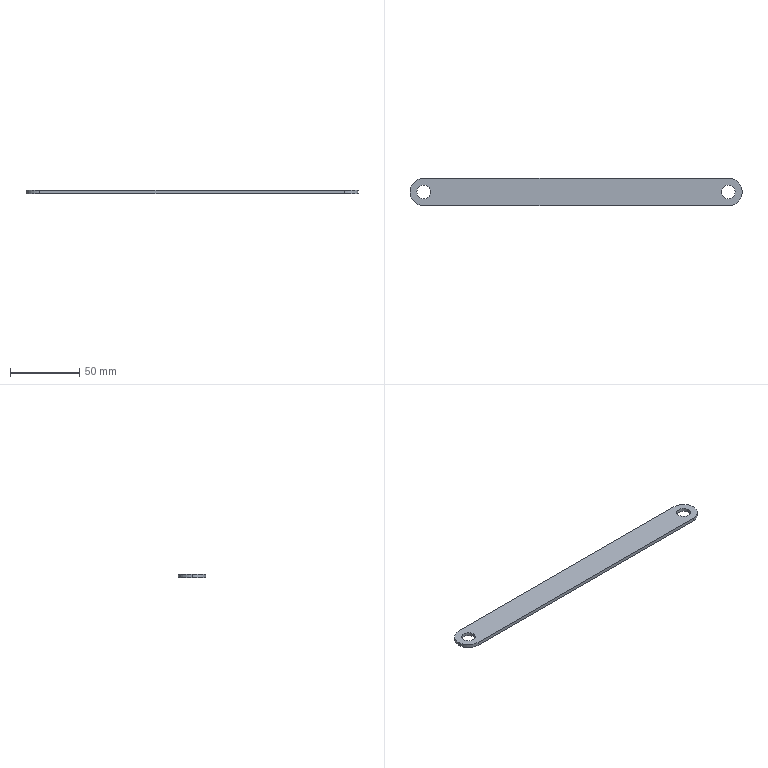Part | SolidWorks | features Extrusion 1 | 1 solid | 11 faces | box 240 x 20 x 2.5 mm | volume 11393 mm3 | cylinder 7 | plane 4 | commonest cylinder face diameters 10 x4 20 x3
STEP:
#1=CARTESIAN_POINT('',(105.,0.,2.5));
#2=VERTEX_POINT('',#1);
#3=CARTESIAN_POINT('',(115.,0.,2.5));
#4=VERTEX_POINT('',#3);
#5=CARTESIAN_POINT('',(110.,0.,2.5));
#6=DIRECTION('',(0.,0.,1.));
#7=DIRECTION('',(1.,0.,0.));
#8=AXIS2_PLACEMENT_3D('',#5,#6,#7);
#9=CIRCLE('',#8,5.);
#10=EDGE_CURVE('',#2,#4,#9,.T.);
#11=ORIENTED_EDGE('',*,*,#10,.T.);
#12=CARTESIAN_POINT('',(115.,0.,0.));
#13=VERTEX_POINT('',#12);
#14=CARTESIAN_POINT('',(115.,0.,2.5));
#15=DIRECTION('',(0.,0.,-1.));
#16=VECTOR('',#15,1000.);
#17=LINE('',#14,#16);
#18=EDGE_CURVE('',#4,#13,#17,.T.);
#19=ORIENTED_EDGE('',*,*,#18,.T.);
#20=CARTESIAN_POINT('',(105.,0.,0.));
#21=VERTEX_POINT('',#20);
#22=CARTESIAN_POINT('',(110.,0.,0.));
#23=DIRECTION('',(0.,0.,1.));
#24=DIRECTION('',(1.,0.,0.));
#25=AXIS2_PLACEMENT_3D('',#22,#23,#24);
#26=CIRCLE('',#25,5.);
#27=EDGE_CURVE('',#21,#13,#26,.T.);
#28=ORIENTED_EDGE('',*,*,#27,.F.);
#29=CARTESIAN_POINT('',(105.,0.,2.5));
#30=DIRECTION('',(0.,0.,-1.));
#31=VECTOR('',#30,1000.);
#32=LINE('',#29,#31);
#33=EDGE_CURVE('',#2,#21,#32,.T.);
#34=ORIENTED_EDGE('',*,*,#33,.F.);
#35=EDGE_LOOP('',(#11,#19,#28,#34));
#36=FACE_OUTER_BOUND('',#35,.T.);
#37=CARTESIAN_POINT('',(110.,0.,2.5));
#38=DIRECTION('',(0.,0.,-1.));
#39=DIRECTION('',(-1.,0.,0.));
#40=AXIS2_PLACEMENT_3D('',#37,#38,#39);
#41=CYLINDRICAL_SURFACE('',#40,5.);
#42=ADVANCED_FACE('',(#36),#41,.F.);
#43=CARTESIAN_POINT('',(-115.,0.,2.5));
#44=VERTEX_POINT('',#43);
#45=CARTESIAN_POINT('',(-105.,0.,2.5));
#46=VERTEX_POINT('',#45);
#47=CARTESIAN_POINT('',(-110.,0.,2.5));
#48=DIRECTION('',(0.,0.,1.));
#49=DIRECTION('',(1.,0.,0.));
#50=AXIS2_PLACEMENT_3D('',#47,#48,#49);
#51=CIRCLE('',#50,5.);
#52=EDGE_CURVE('',#44,#46,#51,.T.);
#53=ORIENTED_EDGE('',*,*,#52,.T.);
#54=CARTESIAN_POINT('',(-105.,0.,0.));
#55=VERTEX_POINT('',#54);
#56=CARTESIAN_POINT('',(-105.,0.,2.5));
#57=DIRECTION('',(0.,0.,-1.));
#58=VECTOR('',#57,1000.);
#59=LINE('',#56,#58);
#60=EDGE_CURVE('',#46,#55,#59,.T.);
#61=ORIENTED_EDGE('',*,*,#60,.T.);
#62=CARTESIAN_POINT('',(-115.,0.,0.));
#63=VERTEX_POINT('',#62);
#64=CARTESIAN_POINT('',(-110.,0.,0.));
#65=DIRECTION('',(0.,0.,1.));
#66=DIRECTION('',(1.,0.,0.));
#67=AXIS2_PLACEMENT_3D('',#64,#65,#66);
#68=CIRCLE('',#67,5.);
#69=EDGE_CURVE('',#63,#55,#68,.T.);
#70=ORIENTED_EDGE('',*,*,#69,.F.);
#71=CARTESIAN_POINT('',(-115.,0.,2.5));
#72=DIRECTION('',(0.,0.,-1.));
#73=VECTOR('',#72,1000.);
#74=LINE('',#71,#73);
#75=EDGE_CURVE('',#44,#63,#74,.T.);
#76=ORIENTED_EDGE('',*,*,#75,.F.);
#77=EDGE_LOOP('',(#53,#61,#70,#76));
#78=FACE_OUTER_BOUND('',#77,.T.);
#79=CARTESIAN_POINT('',(-110.,0.,2.5));
#80=DIRECTION('',(0.,0.,-1.));
#81=DIRECTION('',(-1.,0.,0.));
#82=AXIS2_PLACEMENT_3D('',#79,#80,#81);
#83=CYLINDRICAL_SURFACE('',#82,5.);
#84=ADVANCED_FACE('',(#78),#83,.F.);
#85=CARTESIAN_POINT('',(-120.,0.,2.5));
#86=VERTEX_POINT('',#85);
#87=CARTESIAN_POINT('',(-110.,-10.,2.5));
#88=VERTEX_POINT('',#87);
#89=CARTESIAN_POINT('',(-110.,0.,2.5));
#90=DIRECTION('',(0.,0.,1.));
#91=DIRECTION('',(1.,0.,0.));
#92=AXIS2_PLACEMENT_3D('',#89,#90,#91);
#93=CIRCLE('',#92,10.);
#94=EDGE_CURVE('',#86,#88,#93,.T.);
#95=ORIENTED_EDGE('',*,*,#94,.F.);
#96=CARTESIAN_POINT('',(-120.,0.,0.));
#97=VERTEX_POINT('',#96);
#98=CARTESIAN_POINT('',(-120.,0.,2.5));
#99=DIRECTION('',(0.,0.,-1.));
#100=VECTOR('',#99,1000.);
#101=LINE('',#98,#100);
#102=EDGE_CURVE('',#86,#97,#101,.T.);
#103=ORIENTED_EDGE('',*,*,#102,.T.);
#104=CARTESIAN_POINT('',(-110.,-10.,0.));
#105=VERTEX_POINT('',#104);
#106=CARTESIAN_POINT('',(-110.,0.,0.));
#107=DIRECTION('',(0.,0.,1.));
#108=DIRECTION('',(1.,0.,0.));
#109=AXIS2_PLACEMENT_3D('',#106,#107,#108);
#110=CIRCLE('',#109,10.);
#111=EDGE_CURVE('',#97,#105,#110,.T.);
#112=ORIENTED_EDGE('',*,*,#111,.T.);
#113=CARTESIAN_POINT('',(-110.,-10.,2.5));
#114=DIRECTION('',(0.,0.,-1.));
#115=VECTOR('',#114,1000.);
#116=LINE('',#113,#115);
#117=EDGE_CURVE('',#88,#105,#116,.T.);
#118=ORIENTED_EDGE('',*,*,#117,.F.);
#119=EDGE_LOOP('',(#95,#103,#112,#118));
#120=FACE_OUTER_BOUND('',#119,.T.);
#121=CARTESIAN_POINT('',(-110.,0.,2.5));
#122=DIRECTION('',(0.,0.,-1.));
#123=DIRECTION('',(-1.,0.,0.));
#124=AXIS2_PLACEMENT_3D('',#121,#122,#123);
#125=CYLINDRICAL_SURFACE('',#124,10.);
#126=ADVANCED_FACE('',(#120),#125,.T.);
#127=ORIENTED_EDGE('',*,*,#52,.F.);
#128=CARTESIAN_POINT('',(-110.,0.,2.5));
#129=DIRECTION('',(0.,0.,1.));
#130=DIRECTION('',(1.,0.,0.));
#131=AXIS2_PLACEMENT_3D('',#128,#129,#130);
#132=CIRCLE('',#131,5.);
#133=EDGE_CURVE('',#46,#44,#132,.T.);
#134=ORIENTED_EDGE('',*,*,#133,.F.);
#135=EDGE_LOOP('',(#127,#134));
#136=FACE_BOUND('',#135,.T.);
#137=CARTESIAN_POINT('',(-110.,10.,2.5));
#138=VERTEX_POINT('',#137);
#139=CARTESIAN_POINT('',(-110.,0.,2.5));
#140=DIRECTION('',(0.,0.,1.));
#141=DIRECTION('',(1.,0.,0.));
#142=AXIS2_PLACEMENT_3D('',#139,#140,#141);
#143=CIRCLE('',#142,10.);
#144=EDGE_CURVE('',#138,#86,#143,.T.);
#145=ORIENTED_EDGE('',*,*,#144,.T.);
#146=ORIENTED_EDGE('',*,*,#94,.T.);
#147=CARTESIAN_POINT('',(110.,-10.,2.5));
#148=VERTEX_POINT('',#147);
#149=CARTESIAN_POINT('',(-110.,-10.,2.5));
#150=DIRECTION('',(1.,0.,0.));
#151=VECTOR('',#150,1000.);
#152=LINE('',#149,#151);
#153=EDGE_CURVE('',#88,#148,#152,.T.);
#154=ORIENTED_EDGE('',*,*,#153,.T.);
#155=CARTESIAN_POINT('',(110.,10.,2.5));
#156=VERTEX_POINT('',#155);
#157=CARTESIAN_POINT('',(110.,0.,2.5));
#158=DIRECTION('',(0.,0.,1.));
#159=DIRECTION('',(1.,0.,0.));
#160=AXIS2_PLACEMENT_3D('',#157,#158,#159);
#161=CIRCLE('',#160,10.);
#162=EDGE_CURVE('',#148,#156,#161,.T.);
#163=ORIENTED_EDGE('',*,*,#162,.T.);
#164=CARTESIAN_POINT('',(-110.,10.,2.5));
#165=DIRECTION('',(-1.,0.,0.));
#166=VECTOR('',#165,1000.);
#167=LINE('',#164,#166);
#168=EDGE_CURVE('',#156,#138,#167,.T.);
#169=ORIENTED_EDGE('',*,*,#168,.T.);
#170=EDGE_LOOP('',(#145,#146,#154,#163,#169));
#171=FACE_OUTER_BOUND('',#170,.T.);
#172=ORIENTED_EDGE('',*,*,#10,.F.);
#173=CARTESIAN_POINT('',(110.,0.,2.5));
#174=DIRECTION('',(0.,0.,1.));
#175=DIRECTION('',(1.,0.,0.));
#176=AXIS2_PLACEMENT_3D('',#173,#174,#175);
#177=CIRCLE('',#176,5.);
#178=EDGE_CURVE('',#4,#2,#177,.T.);
#179=ORIENTED_EDGE('',*,*,#178,.F.);
#180=EDGE_LOOP('',(#172,#179));
#181=FACE_BOUND('',#180,.T.);
#182=CARTESIAN_POINT('',(-110.,0.,2.5));
#183=DIRECTION('',(0.,0.,1.));
#184=DIRECTION('',(1.,0.,0.));
#185=AXIS2_PLACEMENT_3D('',#182,#183,#184);
#186=PLANE('',#185);
#187=ADVANCED_FACE('',(#136,#171,#181),#186,.T.);
#188=CARTESIAN_POINT('',(-110.,10.,0.));
#189=VERTEX_POINT('',#188);
#190=CARTESIAN_POINT('',(-110.,0.,0.));
#191=DIRECTION('',(0.,0.,1.));
#192=DIRECTION('',(1.,0.,0.));
#193=AXIS2_PLACEMENT_3D('',#190,#191,#192);
#194=CIRCLE('',#193,10.);
#195=EDGE_CURVE('',#189,#97,#194,.T.);
#196=ORIENTED_EDGE('',*,*,#195,.F.);
#197=CARTESIAN_POINT('',(110.,10.,0.));
#198=VERTEX_POINT('',#197);
#199=CARTESIAN_POINT('',(-110.,10.,0.));
#200=DIRECTION('',(-1.,0.,0.));
#201=VECTOR('',#200,1000.);
#202=LINE('',#199,#201);
#203=EDGE_CURVE('',#198,#189,#202,.T.);
#204=ORIENTED_EDGE('',*,*,#203,.F.);
#205=CARTESIAN_POINT('',(110.,-10.,0.));
#206=VERTEX_POINT('',#205);
#207=CARTESIAN_POINT('',(110.,0.,0.));
#208=DIRECTION('',(0.,0.,1.));
#209=DIRECTION('',(1.,0.,0.));
#210=AXIS2_PLACEMENT_3D('',#207,#208,#209);
#211=CIRCLE('',#210,10.);
#212=EDGE_CURVE('',#206,#198,#211,.T.);
#213=ORIENTED_EDGE('',*,*,#212,.F.);
#214=CARTESIAN_POINT('',(-110.,-10.,0.));
#215=DIRECTION('',(1.,0.,0.));
#216=VECTOR('',#215,1000.);
#217=LINE('',#214,#216);
#218=EDGE_CURVE('',#105,#206,#217,.T.);
#219=ORIENTED_EDGE('',*,*,#218,.F.);
#220=ORIENTED_EDGE('',*,*,#111,.F.);
#221=EDGE_LOOP('',(#196,#204,#213,#219,#220));
#222=FACE_OUTER_BOUND('',#221,.T.);
#223=ORIENTED_EDGE('',*,*,#69,.T.);
#224=CARTESIAN_POINT('',(-110.,0.,0.));
#225=DIRECTION('',(0.,0.,1.));
#226=DIRECTION('',(1.,0.,0.));
#227=AXIS2_PLACEMENT_3D('',#224,#225,#226);
#228=CIRCLE('',#227,5.);
#229=EDGE_CURVE('',#55,#63,#228,.T.);
#230=ORIENTED_EDGE('',*,*,#229,.T.);
#231=EDGE_LOOP('',(#223,#230));
#232=FACE_BOUND('',#231,.T.);
#233=ORIENTED_EDGE('',*,*,#27,.T.);
#234=CARTESIAN_POINT('',(110.,0.,0.));
#235=DIRECTION('',(0.,0.,1.));
#236=DIRECTION('',(1.,0.,0.));
#237=AXIS2_PLACEMENT_3D('',#234,#235,#236);
#238=CIRCLE('',#237,5.);
#239=EDGE_CURVE('',#13,#21,#238,.T.);
#240=ORIENTED_EDGE('',*,*,#239,.T.);
#241=EDGE_LOOP('',(#233,#240));
#242=FACE_BOUND('',#241,.T.);
#243=CARTESIAN_POINT('',(-110.,0.,0.));
#244=DIRECTION('',(0.,0.,1.));
#245=DIRECTION('',(1.,0.,0.));
#246=AXIS2_PLACEMENT_3D('',#243,#244,#245);
#247=PLANE('',#246);
#248=ADVANCED_FACE('',(#222,#232,#242),#247,.F.);
#249=ORIENTED_EDGE('',*,*,#102,.F.);
#250=ORIENTED_EDGE('',*,*,#144,.F.);
#251=CARTESIAN_POINT('',(-110.,10.,2.5));
#252=DIRECTION('',(0.,0.,-1.));
#253=VECTOR('',#252,1000.);
#254=LINE('',#251,#253);
#255=EDGE_CURVE('',#138,#189,#254,.T.);
#256=ORIENTED_EDGE('',*,*,#255,.T.);
#257=ORIENTED_EDGE('',*,*,#195,.T.);
#258=EDGE_LOOP('',(#249,#250,#256,#257));
#259=FACE_OUTER_BOUND('',#258,.T.);
#260=CARTESIAN_POINT('',(-110.,0.,2.5));
#261=DIRECTION('',(0.,0.,-1.));
#262=DIRECTION('',(-1.,0.,0.));
#263=AXIS2_PLACEMENT_3D('',#260,#261,#262);
#264=CYLINDRICAL_SURFACE('',#263,10.);
#265=ADVANCED_FACE('',(#259),#264,.T.);
#266=ORIENTED_EDGE('',*,*,#218,.T.);
#267=CARTESIAN_POINT('',(110.,-10.,2.5));
#268=DIRECTION('',(0.,0.,-1.));
#269=VECTOR('',#268,1000.);
#270=LINE('',#267,#269);
#271=EDGE_CURVE('',#148,#206,#270,.T.);
#272=ORIENTED_EDGE('',*,*,#271,.F.);
#273=ORIENTED_EDGE('',*,*,#153,.F.);
#274=ORIENTED_EDGE('',*,*,#117,.T.);
#275=EDGE_LOOP('',(#266,#272,#273,#274));
#276=FACE_OUTER_BOUND('',#275,.T.);
#277=CARTESIAN_POINT('',(-110.,-10.,2.5));
#278=DIRECTION('',(0.,1.,0.));
#279=DIRECTION('',(0.,0.,1.));
#280=AXIS2_PLACEMENT_3D('',#277,#278,#279);
#281=PLANE('',#280);
#282=ADVANCED_FACE('',(#276),#281,.F.);
#283=ORIENTED_EDGE('',*,*,#212,.T.);
#284=CARTESIAN_POINT('',(110.,10.,2.5));
#285=DIRECTION('',(0.,0.,-1.));
#286=VECTOR('',#285,1000.);
#287=LINE('',#284,#286);
#288=EDGE_CURVE('',#156,#198,#287,.T.);
#289=ORIENTED_EDGE('',*,*,#288,.F.);
#290=ORIENTED_EDGE('',*,*,#162,.F.);
#291=ORIENTED_EDGE('',*,*,#271,.T.);
#292=EDGE_LOOP('',(#283,#289,#290,#291));
#293=FACE_OUTER_BOUND('',#292,.T.);
#294=CARTESIAN_POINT('',(110.,0.,2.5));
#295=DIRECTION('',(0.,0.,-1.));
#296=DIRECTION('',(-1.,0.,0.));
#297=AXIS2_PLACEMENT_3D('',#294,#295,#296);
#298=CYLINDRICAL_SURFACE('',#297,10.);
#299=ADVANCED_FACE('',(#293),#298,.T.);
#300=ORIENTED_EDGE('',*,*,#203,.T.);
#301=ORIENTED_EDGE('',*,*,#255,.F.);
#302=ORIENTED_EDGE('',*,*,#168,.F.);
#303=ORIENTED_EDGE('',*,*,#288,.T.);
#304=EDGE_LOOP('',(#300,#301,#302,#303));
#305=FACE_OUTER_BOUND('',#304,.T.);
#306=CARTESIAN_POINT('',(-110.,10.,2.5));
#307=DIRECTION('',(0.,-1.,0.));
#308=DIRECTION('',(0.,0.,-1.));
#309=AXIS2_PLACEMENT_3D('',#306,#307,#308);
#310=PLANE('',#309);
#311=ADVANCED_FACE('',(#305),#310,.F.);
#312=ORIENTED_EDGE('',*,*,#60,.F.);
#313=ORIENTED_EDGE('',*,*,#133,.T.);
#314=ORIENTED_EDGE('',*,*,#75,.T.);
#315=ORIENTED_EDGE('',*,*,#229,.F.);
#316=EDGE_LOOP('',(#312,#313,#314,#315));
#317=FACE_OUTER_BOUND('',#316,.T.);
#318=CARTESIAN_POINT('',(-110.,0.,2.5));
#319=DIRECTION('',(0.,0.,-1.));
#320=DIRECTION('',(-1.,0.,0.));
#321=AXIS2_PLACEMENT_3D('',#318,#319,#320);
#322=CYLINDRICAL_SURFACE('',#321,5.);
#323=ADVANCED_FACE('',(#317),#322,.F.);
#324=ORIENTED_EDGE('',*,*,#18,.F.);
#325=ORIENTED_EDGE('',*,*,#178,.T.);
#326=ORIENTED_EDGE('',*,*,#33,.T.);
#327=ORIENTED_EDGE('',*,*,#239,.F.);
#328=EDGE_LOOP('',(#324,#325,#326,#327));
#329=FACE_OUTER_BOUND('',#328,.T.);
#330=CARTESIAN_POINT('',(110.,0.,2.5));
#331=DIRECTION('',(0.,0.,-1.));
#332=DIRECTION('',(-1.,0.,0.));
#333=AXIS2_PLACEMENT_3D('',#330,#331,#332);
#334=CYLINDRICAL_SURFACE('',#333,5.);
#335=ADVANCED_FACE('',(#329),#334,.F.);
#336=CLOSED_SHELL('',(#42,#84,#126,#187,#248,#265,#282,#299,#311,#323,#335));
#337=MANIFOLD_SOLID_BREP('',#336);
#338=CARTESIAN_POINT('',(0.,0.,0.));
#339=DIRECTION('',(0.,0.,1.));
#340=DIRECTION('',(1.,0.,0.));
#341=AXIS2_PLACEMENT_3D('',#338,#339,#340);
#342=(LENGTH_UNIT()NAMED_UNIT(*)SI_UNIT(.MILLI.,.METRE.));
#343=UNCERTAINTY_MEASURE_WITH_UNIT(LENGTH_MEASURE(0.00001),#342,'','');
#344=(NAMED_UNIT(*)PLANE_ANGLE_UNIT()SI_UNIT($,.RADIAN.));
#345=(NAMED_UNIT(*)SI_UNIT($,.STERADIAN.)SOLID_ANGLE_UNIT());
#346=(GEOMETRIC_REPRESENTATION_CONTEXT(3)GLOBAL_UNCERTAINTY_ASSIGNED_CONTEXT((#343))GLOBAL_UNIT_ASSIGNED_CONTEXT((#342,#344,#345))REPRESENTATION_CONTEXT('',''));
#347=ADVANCED_BREP_SHAPE_REPRESENTATION('',(#337,#341),#346);